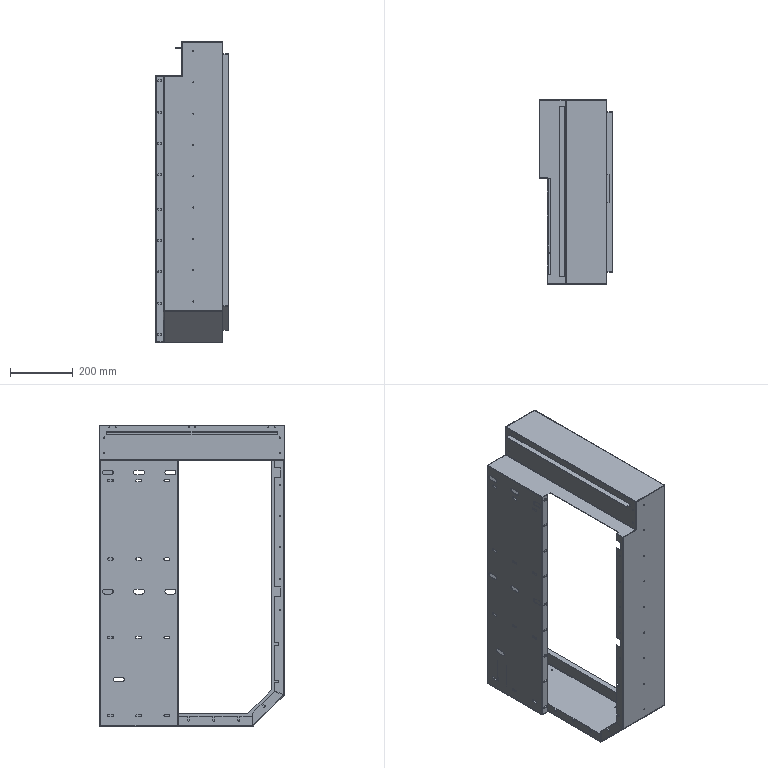Part | SolidWorks | features HoleWzd 15, FlatPattern 7, ICE 7, SheetMetal 7, SolidToSheetMetal 6, Cut 5, EdgeFlange 3, Chamfer 1, Extrusion 1, SMBaseFlange 1 | 8 solids | 372 faces | box 233 x 588 x 960 mm | volume 1652161 mm3 | plane 225 | cylinder 142 | spline 5 | commonest cylinder face diameters 7 x48 3.3 x30 4.2 x18 15 x14 1.473 x11 4.473 x11